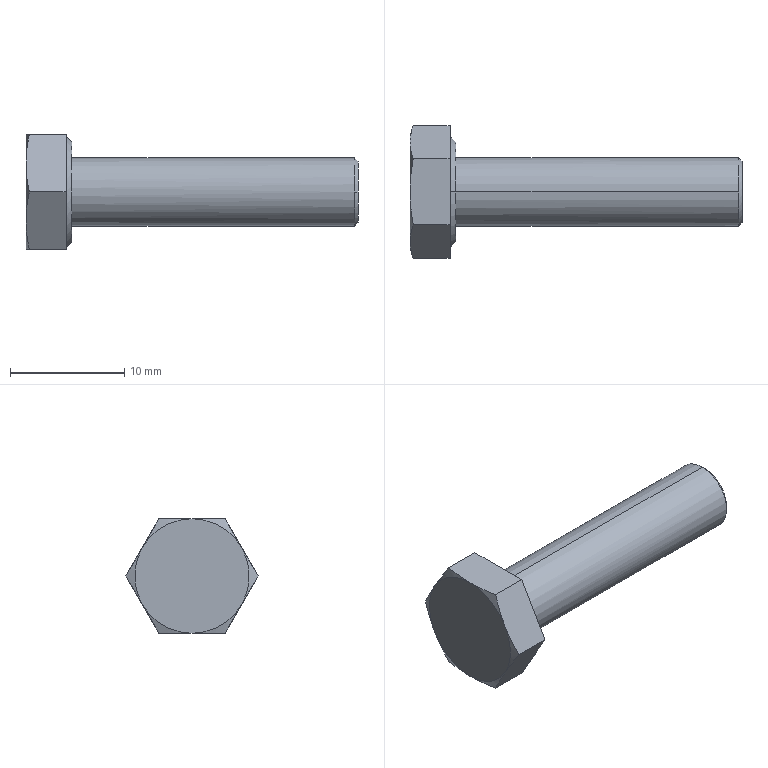Part | STEP file | hex head bolts-full thread grade c gb_GB_FASTENER_BOLT_HHBFTC M6X25-S | 1 solid | 22 faces | box 29 x 11.547 x 10 mm | volume 1042 mm3 | cone 10 | plane 10 | cylinder 2 | commonest cylinder face diameters 6 x2
STEP:
#1=CARTESIAN_POINT('',(28.7,3.,0.));
#2=VERTEX_POINT('',#1);
#3=CARTESIAN_POINT('',(28.7,0.,-3.));
#4=VERTEX_POINT('',#3);
#5=CARTESIAN_POINT('',(28.7,0.,0.));
#6=DIRECTION('',(-1.,0.,0.));
#7=DIRECTION('',(0.,0.,1.));
#8=AXIS2_PLACEMENT_3D('',#5,#6,#7);
#9=CIRCLE('',#8,3.);
#10=EDGE_CURVE('',#2,#4,#9,.T.);
#11=ORIENTED_EDGE('',*,*,#10,.T.);
#12=CARTESIAN_POINT('',(4.,0.,-3.));
#13=VERTEX_POINT('',#12);
#14=CARTESIAN_POINT('',(29.,0.,-3.));
#15=DIRECTION('',(-1.,0.,0.));
#16=VECTOR('',#15,1000.);
#17=LINE('',#14,#16);
#18=EDGE_CURVE('',#4,#13,#17,.T.);
#19=ORIENTED_EDGE('',*,*,#18,.T.);
#20=CARTESIAN_POINT('',(4.,0.,3.));
#21=VERTEX_POINT('',#20);
#22=CARTESIAN_POINT('',(4.,0.,0.));
#23=DIRECTION('',(1.,0.,0.));
#24=DIRECTION('',(0.,0.,1.));
#25=AXIS2_PLACEMENT_3D('',#22,#23,#24);
#26=CIRCLE('',#25,3.);
#27=EDGE_CURVE('',#13,#21,#26,.T.);
#28=ORIENTED_EDGE('',*,*,#27,.T.);
#29=CARTESIAN_POINT('',(28.7,0.,3.));
#30=VERTEX_POINT('',#29);
#31=CARTESIAN_POINT('',(29.,0.,3.));
#32=DIRECTION('',(-1.,0.,0.));
#33=VECTOR('',#32,1000.);
#34=LINE('',#31,#33);
#35=EDGE_CURVE('',#30,#21,#34,.T.);
#36=ORIENTED_EDGE('',*,*,#35,.F.);
#37=CARTESIAN_POINT('',(28.7,0.,0.));
#38=DIRECTION('',(-1.,0.,0.));
#39=DIRECTION('',(0.,0.,1.));
#40=AXIS2_PLACEMENT_3D('',#37,#38,#39);
#41=CIRCLE('',#40,3.);
#42=EDGE_CURVE('',#30,#2,#41,.T.);
#43=ORIENTED_EDGE('',*,*,#42,.T.);
#44=EDGE_LOOP('',(#11,#19,#28,#36,#43));
#45=FACE_OUTER_BOUND('',#44,.T.);
#46=CARTESIAN_POINT('',(29.,0.,0.));
#47=DIRECTION('',(-1.,0.,0.));
#48=DIRECTION('',(0.,0.,1.));
#49=AXIS2_PLACEMENT_3D('',#46,#47,#48);
#50=CYLINDRICAL_SURFACE('',#49,3.);
#51=ADVANCED_FACE('',(#45),#50,.T.);
#52=CARTESIAN_POINT('',(29.,-2.7,0.));
#53=VERTEX_POINT('',#52);
#54=CARTESIAN_POINT('',(29.,2.7,0.));
#55=VERTEX_POINT('',#54);
#56=CARTESIAN_POINT('',(29.,0.,0.));
#57=DIRECTION('',(-1.,0.,0.));
#58=DIRECTION('',(0.,-1.,0.));
#59=AXIS2_PLACEMENT_3D('',#56,#57,#58);
#60=CIRCLE('',#59,2.7);
#61=EDGE_CURVE('',#53,#55,#60,.T.);
#62=ORIENTED_EDGE('',*,*,#61,.T.);
#63=CARTESIAN_POINT('',(28.7,3.,0.));
#64=DIRECTION('',(-0.7071,0.7071,0.));
#65=VECTOR('',#64,1000.);
#66=LINE('',#63,#65);
#67=EDGE_CURVE('',#55,#2,#66,.T.);
#68=ORIENTED_EDGE('',*,*,#67,.T.);
#69=ORIENTED_EDGE('',*,*,#42,.F.);
#70=CARTESIAN_POINT('',(28.7,-3.,0.));
#71=VERTEX_POINT('',#70);
#72=CARTESIAN_POINT('',(28.7,0.,0.));
#73=DIRECTION('',(-1.,0.,0.));
#74=DIRECTION('',(0.,0.,1.));
#75=AXIS2_PLACEMENT_3D('',#72,#73,#74);
#76=CIRCLE('',#75,3.);
#77=EDGE_CURVE('',#71,#30,#76,.T.);
#78=ORIENTED_EDGE('',*,*,#77,.F.);
#79=CARTESIAN_POINT('',(28.7,-3.,0.));
#80=DIRECTION('',(-0.7071,-0.7071,0.));
#81=VECTOR('',#80,1000.);
#82=LINE('',#79,#81);
#83=EDGE_CURVE('',#53,#71,#82,.T.);
#84=ORIENTED_EDGE('',*,*,#83,.F.);
#85=EDGE_LOOP('',(#62,#68,#69,#78,#84));
#86=FACE_OUTER_BOUND('',#85,.T.);
#87=CARTESIAN_POINT('',(28.7,0.,0.));
#88=DIRECTION('',(-1.,0.,0.));
#89=DIRECTION('',(0.,-1.,0.));
#90=AXIS2_PLACEMENT_3D('',#87,#88,#89);
#91=CONICAL_SURFACE('',#90,3.,0.7854);
#92=ADVANCED_FACE('',(#86),#91,.T.);
#93=CARTESIAN_POINT('',(4.,0.,4.37));
#94=VERTEX_POINT('',#93);
#95=CARTESIAN_POINT('',(4.,0.,-4.37));
#96=VERTEX_POINT('',#95);
#97=CARTESIAN_POINT('',(4.,0.,0.));
#98=DIRECTION('',(-1.,0.,0.));
#99=DIRECTION('',(0.,0.,1.));
#100=AXIS2_PLACEMENT_3D('',#97,#98,#99);
#101=CIRCLE('',#100,4.37);
#102=EDGE_CURVE('',#94,#96,#101,.T.);
#103=ORIENTED_EDGE('',*,*,#102,.T.);
#104=CARTESIAN_POINT('',(3.5,0.,-4.87));
#105=VERTEX_POINT('',#104);
#106=CARTESIAN_POINT('',(3.5,0.,-4.87));
#107=DIRECTION('',(-0.7071,0.,-0.7071));
#108=VECTOR('',#107,1000.);
#109=LINE('',#106,#108);
#110=EDGE_CURVE('',#96,#105,#109,.T.);
#111=ORIENTED_EDGE('',*,*,#110,.T.);
#112=CARTESIAN_POINT('',(3.5,0.,4.87));
#113=VERTEX_POINT('',#112);
#114=CARTESIAN_POINT('',(3.5,0.,0.));
#115=DIRECTION('',(1.,0.,0.));
#116=DIRECTION('',(0.,0.,1.));
#117=AXIS2_PLACEMENT_3D('',#114,#115,#116);
#118=CIRCLE('',#117,4.87);
#119=EDGE_CURVE('',#105,#113,#118,.T.);
#120=ORIENTED_EDGE('',*,*,#119,.T.);
#121=CARTESIAN_POINT('',(3.5,0.,4.87));
#122=DIRECTION('',(-0.7071,0.,0.7071));
#123=VECTOR('',#122,1000.);
#124=LINE('',#121,#123);
#125=EDGE_CURVE('',#94,#113,#124,.T.);
#126=ORIENTED_EDGE('',*,*,#125,.F.);
#127=EDGE_LOOP('',(#103,#111,#120,#126));
#128=FACE_OUTER_BOUND('',#127,.T.);
#129=CARTESIAN_POINT('',(3.5,0.,0.));
#130=DIRECTION('',(-1.,0.,0.));
#131=DIRECTION('',(0.,0.,1.));
#132=AXIS2_PLACEMENT_3D('',#129,#130,#131);
#133=CONICAL_SURFACE('',#132,4.87,0.7854);
#134=ADVANCED_FACE('',(#128),#133,.T.);
#135=ORIENTED_EDGE('',*,*,#18,.F.);
#136=CARTESIAN_POINT('',(28.7,0.,0.));
#137=DIRECTION('',(-1.,0.,0.));
#138=DIRECTION('',(0.,0.,1.));
#139=AXIS2_PLACEMENT_3D('',#136,#137,#138);
#140=CIRCLE('',#139,3.);
#141=EDGE_CURVE('',#4,#71,#140,.T.);
#142=ORIENTED_EDGE('',*,*,#141,.T.);
#143=ORIENTED_EDGE('',*,*,#77,.T.);
#144=ORIENTED_EDGE('',*,*,#35,.T.);
#145=CARTESIAN_POINT('',(4.,0.,0.));
#146=DIRECTION('',(1.,0.,0.));
#147=DIRECTION('',(0.,0.,1.));
#148=AXIS2_PLACEMENT_3D('',#145,#146,#147);
#149=CIRCLE('',#148,3.);
#150=EDGE_CURVE('',#21,#13,#149,.T.);
#151=ORIENTED_EDGE('',*,*,#150,.T.);
#152=EDGE_LOOP('',(#135,#142,#143,#144,#151));
#153=FACE_OUTER_BOUND('',#152,.T.);
#154=CARTESIAN_POINT('',(29.,0.,0.));
#155=DIRECTION('',(-1.,0.,0.));
#156=DIRECTION('',(0.,0.,1.));
#157=AXIS2_PLACEMENT_3D('',#154,#155,#156);
#158=CYLINDRICAL_SURFACE('',#157,3.);
#159=ADVANCED_FACE('',(#153),#158,.T.);
#160=ORIENTED_EDGE('',*,*,#150,.F.);
#161=ORIENTED_EDGE('',*,*,#27,.F.);
#162=EDGE_LOOP('',(#160,#161));
#163=FACE_BOUND('',#162,.T.);
#164=ORIENTED_EDGE('',*,*,#102,.F.);
#165=CARTESIAN_POINT('',(4.,0.,0.));
#166=DIRECTION('',(-1.,0.,0.));
#167=DIRECTION('',(0.,0.,1.));
#168=AXIS2_PLACEMENT_3D('',#165,#166,#167);
#169=CIRCLE('',#168,4.37);
#170=EDGE_CURVE('',#96,#94,#169,.T.);
#171=ORIENTED_EDGE('',*,*,#170,.F.);
#172=EDGE_LOOP('',(#164,#171));
#173=FACE_OUTER_BOUND('',#172,.T.);
#174=CARTESIAN_POINT('',(4.,0.,10.));
#175=DIRECTION('',(-1.,0.,0.));
#176=DIRECTION('',(0.,0.,1.));
#177=AXIS2_PLACEMENT_3D('',#174,#175,#176);
#178=PLANE('',#177);
#179=ADVANCED_FACE('',(#163,#173),#178,.F.);
#180=ORIENTED_EDGE('',*,*,#67,.F.);
#181=CARTESIAN_POINT('',(29.,0.,0.));
#182=DIRECTION('',(-1.,0.,0.));
#183=DIRECTION('',(0.,-1.,0.));
#184=AXIS2_PLACEMENT_3D('',#181,#182,#183);
#185=CIRCLE('',#184,2.7);
#186=EDGE_CURVE('',#55,#53,#185,.T.);
#187=ORIENTED_EDGE('',*,*,#186,.T.);
#188=ORIENTED_EDGE('',*,*,#83,.T.);
#189=ORIENTED_EDGE('',*,*,#141,.F.);
#190=ORIENTED_EDGE('',*,*,#10,.F.);
#191=EDGE_LOOP('',(#180,#187,#188,#189,#190));
#192=FACE_OUTER_BOUND('',#191,.T.);
#193=CARTESIAN_POINT('',(28.7,0.,0.));
#194=DIRECTION('',(-1.,0.,0.));
#195=DIRECTION('',(0.,-1.,0.));
#196=AXIS2_PLACEMENT_3D('',#193,#194,#195);
#197=CONICAL_SURFACE('',#196,3.,0.7854);
#198=ADVANCED_FACE('',(#192),#197,.T.);
#199=ORIENTED_EDGE('',*,*,#110,.F.);
#200=ORIENTED_EDGE('',*,*,#170,.T.);
#201=ORIENTED_EDGE('',*,*,#125,.T.);
#202=CARTESIAN_POINT('',(3.5,0.,0.));
#203=DIRECTION('',(1.,0.,0.));
#204=DIRECTION('',(0.,0.,1.));
#205=AXIS2_PLACEMENT_3D('',#202,#203,#204);
#206=CIRCLE('',#205,4.87);
#207=EDGE_CURVE('',#113,#105,#206,.T.);
#208=ORIENTED_EDGE('',*,*,#207,.T.);
#209=EDGE_LOOP('',(#199,#200,#201,#208));
#210=FACE_OUTER_BOUND('',#209,.T.);
#211=CARTESIAN_POINT('',(3.5,0.,0.));
#212=DIRECTION('',(-1.,0.,0.));
#213=DIRECTION('',(0.,0.,1.));
#214=AXIS2_PLACEMENT_3D('',#211,#212,#213);
#215=CONICAL_SURFACE('',#214,4.87,0.7854);
#216=ADVANCED_FACE('',(#210),#215,.T.);
#217=ORIENTED_EDGE('',*,*,#61,.F.);
#218=ORIENTED_EDGE('',*,*,#186,.F.);
#219=EDGE_LOOP('',(#217,#218));
#220=FACE_OUTER_BOUND('',#219,.T.);
#221=CARTESIAN_POINT('',(29.,0.,0.));
#222=DIRECTION('',(1.,0.,0.));
#223=DIRECTION('',(0.,0.,-1.));
#224=AXIS2_PLACEMENT_3D('',#221,#222,#223);
#225=PLANE('',#224);
#226=ADVANCED_FACE('',(#220),#225,.T.);
#227=CARTESIAN_POINT('',(3.5,5.774,0.));
#228=VERTEX_POINT('',#227);
#229=CARTESIAN_POINT('',(3.5,2.887,5.));
#230=VERTEX_POINT('',#229);
#231=CARTESIAN_POINT('',(3.5,5.774,0.));
#232=DIRECTION('',(0.,-0.5,0.866));
#233=VECTOR('',#232,1000.);
#234=LINE('',#231,#233);
#235=EDGE_CURVE('',#228,#230,#234,.T.);
#236=ORIENTED_EDGE('',*,*,#235,.T.);
#237=CARTESIAN_POINT('',(3.5,-2.887,5.));
#238=VERTEX_POINT('',#237);
#239=CARTESIAN_POINT('',(3.5,4.87,5.));
#240=DIRECTION('',(0.,-1.,0.));
#241=VECTOR('',#240,1000.);
#242=LINE('',#239,#241);
#243=EDGE_CURVE('',#230,#238,#242,.T.);
#244=ORIENTED_EDGE('',*,*,#243,.T.);
#245=CARTESIAN_POINT('',(3.5,-5.774,0.));
#246=VERTEX_POINT('',#245);
#247=CARTESIAN_POINT('',(3.5,-2.887,5.));
#248=DIRECTION('',(0.,-0.5,-0.866));
#249=VECTOR('',#248,1000.);
#250=LINE('',#247,#249);
#251=EDGE_CURVE('',#238,#246,#250,.T.);
#252=ORIENTED_EDGE('',*,*,#251,.T.);
#253=CARTESIAN_POINT('',(3.5,-2.887,-5.));
#254=VERTEX_POINT('',#253);
#255=CARTESIAN_POINT('',(3.5,-5.774,0.));
#256=DIRECTION('',(0.,0.5,-0.866));
#257=VECTOR('',#256,1000.);
#258=LINE('',#255,#257);
#259=EDGE_CURVE('',#246,#254,#258,.T.);
#260=ORIENTED_EDGE('',*,*,#259,.T.);
#261=CARTESIAN_POINT('',(3.5,2.887,-5.));
#262=VERTEX_POINT('',#261);
#263=CARTESIAN_POINT('',(3.5,4.87,-5.));
#264=DIRECTION('',(0.,1.,0.));
#265=VECTOR('',#264,1000.);
#266=LINE('',#263,#265);
#267=EDGE_CURVE('',#254,#262,#266,.T.);
#268=ORIENTED_EDGE('',*,*,#267,.T.);
#269=CARTESIAN_POINT('',(3.5,2.887,-5.));
#270=DIRECTION('',(0.,0.5,0.866));
#271=VECTOR('',#270,1000.);
#272=LINE('',#269,#271);
#273=EDGE_CURVE('',#262,#228,#272,.T.);
#274=ORIENTED_EDGE('',*,*,#273,.T.);
#275=EDGE_LOOP('',(#236,#244,#252,#260,#268,#274));
#276=FACE_OUTER_BOUND('',#275,.T.);
#277=ORIENTED_EDGE('',*,*,#207,.F.);
#278=ORIENTED_EDGE('',*,*,#119,.F.);
#279=EDGE_LOOP('',(#277,#278));
#280=FACE_BOUND('',#279,.T.);
#281=CARTESIAN_POINT('',(3.5,4.87,0.));
#282=DIRECTION('',(1.,0.,0.));
#283=DIRECTION('',(0.,0.,-1.));
#284=AXIS2_PLACEMENT_3D('',#281,#282,#283);
#285=PLANE('',#284);
#286=ADVANCED_FACE('',(#276,#280),#285,.T.);
#287=CARTESIAN_POINT('',(0.2815,-2.887,5.));
#288=VERTEX_POINT('',#287);
#289=CARTESIAN_POINT('',(4.,-2.887,5.));
#290=DIRECTION('',(-1.,0.,0.));
#291=VECTOR('',#290,1000.);
#292=LINE('',#289,#291);
#293=EDGE_CURVE('',#238,#288,#292,.T.);
#294=ORIENTED_EDGE('',*,*,#293,.F.);
#295=ORIENTED_EDGE('',*,*,#243,.F.);
#296=CARTESIAN_POINT('',(0.2815,2.887,5.));
#297=VERTEX_POINT('',#296);
#298=CARTESIAN_POINT('',(4.,2.887,5.));
#299=DIRECTION('',(1.,0.,0.));
#300=VECTOR('',#299,1000.);
#301=LINE('',#298,#300);
#302=EDGE_CURVE('',#297,#230,#301,.T.);
#303=ORIENTED_EDGE('',*,*,#302,.F.);
#304=CARTESIAN_POINT('',(0.,0.,5.));
#305=VERTEX_POINT('',#304);
#306=CARTESIAN_POINT('',(0.,0.,5.));
#307=CARTESIAN_POINT('',(0.,0.9714,5.));
#308=CARTESIAN_POINT('',(0.1078,1.932,5.));
#309=CARTESIAN_POINT('',(0.2815,2.887,5.));
#310=B_SPLINE_CURVE_WITH_KNOTS('',3,(#306,#307,#308,#309),.UNSPECIFIED.,.F.,.F.,(4,4),(0.,0.0029),.UNSPECIFIED.);
#311=EDGE_CURVE('',#305,#297,#310,.T.);
#312=ORIENTED_EDGE('',*,*,#311,.F.);
#313=CARTESIAN_POINT('',(0.2815,-2.887,5.));
#314=CARTESIAN_POINT('',(0.1078,-1.932,5.));
#315=CARTESIAN_POINT('',(0.,-0.9714,5.));
#316=CARTESIAN_POINT('',(0.,0.,5.));
#317=B_SPLINE_CURVE_WITH_KNOTS('',3,(#313,#314,#315,#316),.UNSPECIFIED.,.F.,.F.,(4,4),(0.,0.0029),.UNSPECIFIED.);
#318=EDGE_CURVE('',#288,#305,#317,.T.);
#319=ORIENTED_EDGE('',*,*,#318,.F.);
#320=EDGE_LOOP('',(#294,#295,#303,#312,#319));
#321=FACE_OUTER_BOUND('',#320,.T.);
#322=CARTESIAN_POINT('',(4.,2.887,5.));
#323=DIRECTION('',(0.,0.,-1.));
#324=DIRECTION('',(0.,1.,0.));
#325=AXIS2_PLACEMENT_3D('',#322,#323,#324);
#326=PLANE('',#325);
#327=ADVANCED_FACE('',(#321),#326,.F.);
#328=ORIENTED_EDGE('',*,*,#302,.T.);
#329=ORIENTED_EDGE('',*,*,#235,.F.);
#330=CARTESIAN_POINT('',(0.2815,5.774,0.));
#331=VERTEX_POINT('',#330);
#332=CARTESIAN_POINT('',(4.,5.774,0.));
#333=DIRECTION('',(1.,0.,0.));
#334=VECTOR('',#333,1000.);
#335=LINE('',#332,#334);
#336=EDGE_CURVE('',#331,#228,#335,.T.);
#337=ORIENTED_EDGE('',*,*,#336,.F.);
#338=CARTESIAN_POINT('',(0.,4.33,2.5));
#339=VERTEX_POINT('',#338);
#340=CARTESIAN_POINT('',(0.,4.33,2.5));
#341=CARTESIAN_POINT('',(0.,4.816,1.659));
#342=CARTESIAN_POINT('',(0.1078,5.296,0.8266));
#343=CARTESIAN_POINT('',(0.2815,5.774,0.));
#344=B_SPLINE_CURVE_WITH_KNOTS('',3,(#340,#341,#342,#343),.UNSPECIFIED.,.F.,.F.,(4,4),(0.,0.0029),.UNSPECIFIED.);
#345=EDGE_CURVE('',#339,#331,#344,.T.);
#346=ORIENTED_EDGE('',*,*,#345,.F.);
#347=CARTESIAN_POINT('',(0.2815,2.887,5.));
#348=CARTESIAN_POINT('',(0.1078,3.364,4.173));
#349=CARTESIAN_POINT('',(0.,3.844,3.341));
#350=CARTESIAN_POINT('',(0.,4.33,2.5));
#351=B_SPLINE_CURVE_WITH_KNOTS('',3,(#347,#348,#349,#350),.UNSPECIFIED.,.F.,.F.,(4,4),(0.,0.0029),.UNSPECIFIED.);
#352=EDGE_CURVE('',#297,#339,#351,.T.);
#353=ORIENTED_EDGE('',*,*,#352,.F.);
#354=EDGE_LOOP('',(#328,#329,#337,#346,#353));
#355=FACE_OUTER_BOUND('',#354,.T.);
#356=CARTESIAN_POINT('',(4.,5.774,0.));
#357=DIRECTION('',(0.,-0.866,-0.5));
#358=DIRECTION('',(0.,0.5,-0.866));
#359=AXIS2_PLACEMENT_3D('',#356,#357,#358);
#360=PLANE('',#359);
#361=ADVANCED_FACE('',(#355),#360,.F.);
#362=ORIENTED_EDGE('',*,*,#336,.T.);
#363=ORIENTED_EDGE('',*,*,#273,.F.);
#364=CARTESIAN_POINT('',(0.2815,2.887,-5.));
#365=VERTEX_POINT('',#364);
#366=CARTESIAN_POINT('',(4.,2.887,-5.));
#367=DIRECTION('',(1.,0.,0.));
#368=VECTOR('',#367,1000.);
#369=LINE('',#366,#368);
#370=EDGE_CURVE('',#365,#262,#369,.T.);
#371=ORIENTED_EDGE('',*,*,#370,.F.);
#372=CARTESIAN_POINT('',(0.,4.33,-2.5));
#373=VERTEX_POINT('',#372);
#374=CARTESIAN_POINT('',(0.,4.33,-2.5));
#375=CARTESIAN_POINT('',(0.,3.844,-3.341));
#376=CARTESIAN_POINT('',(0.1078,3.364,-4.173));
#377=CARTESIAN_POINT('',(0.2815,2.887,-5.));
#378=B_SPLINE_CURVE_WITH_KNOTS('',3,(#374,#375,#376,#377),.UNSPECIFIED.,.F.,.F.,(4,4),(0.,0.0029),.UNSPECIFIED.);
#379=EDGE_CURVE('',#373,#365,#378,.T.);
#380=ORIENTED_EDGE('',*,*,#379,.F.);
#381=CARTESIAN_POINT('',(0.2815,5.774,0.));
#382=CARTESIAN_POINT('',(0.1078,5.296,-0.8266));
#383=CARTESIAN_POINT('',(0.,4.816,-1.659));
#384=CARTESIAN_POINT('',(0.,4.33,-2.5));
#385=B_SPLINE_CURVE_WITH_KNOTS('',3,(#381,#382,#383,#384),.UNSPECIFIED.,.F.,.F.,(4,4),(0.,0.0029),.UNSPECIFIED.);
#386=EDGE_CURVE('',#331,#373,#385,.T.);
#387=ORIENTED_EDGE('',*,*,#386,.F.);
#388=EDGE_LOOP('',(#362,#363,#371,#380,#387));
#389=FACE_OUTER_BOUND('',#388,.T.);
#390=CARTESIAN_POINT('',(4.,2.887,-5.));
#391=DIRECTION('',(0.,-0.866,0.5));
#392=DIRECTION('',(0.,-0.5,-0.866));
#393=AXIS2_PLACEMENT_3D('',#390,#391,#392);
#394=PLANE('',#393);
#395=ADVANCED_FACE('',(#389),#394,.F.);
#396=ORIENTED_EDGE('',*,*,#370,.T.);
#397=ORIENTED_EDGE('',*,*,#267,.F.);
#398=CARTESIAN_POINT('',(0.2815,-2.887,-5.));
#399=VERTEX_POINT('',#398);
#400=CARTESIAN_POINT('',(4.,-2.887,-5.));
#401=DIRECTION('',(1.,0.,0.));
#402=VECTOR('',#401,1000.);
#403=LINE('',#400,#402);
#404=EDGE_CURVE('',#399,#254,#403,.T.);
#405=ORIENTED_EDGE('',*,*,#404,.F.);
#406=CARTESIAN_POINT('',(0.,0.,-5.));
#407=VERTEX_POINT('',#406);
#408=CARTESIAN_POINT('',(0.,0.,-5.));
#409=CARTESIAN_POINT('',(0.,-0.9714,-5.));
#410=CARTESIAN_POINT('',(0.1078,-1.932,-5.));
#411=CARTESIAN_POINT('',(0.2815,-2.887,-5.));
#412=B_SPLINE_CURVE_WITH_KNOTS('',3,(#408,#409,#410,#411),.UNSPECIFIED.,.F.,.F.,(4,4),(0.,0.0029),.UNSPECIFIED.);
#413=EDGE_CURVE('',#407,#399,#412,.T.);
#414=ORIENTED_EDGE('',*,*,#413,.F.);
#415=CARTESIAN_POINT('',(0.2815,2.887,-5.));
#416=CARTESIAN_POINT('',(0.1078,1.932,-5.));
#417=CARTESIAN_POINT('',(0.,0.9714,-5.));
#418=CARTESIAN_POINT('',(0.,0.,-5.));
#419=B_SPLINE_CURVE_WITH_KNOTS('',3,(#415,#416,#417,#418),.UNSPECIFIED.,.F.,.F.,(4,4),(0.,0.0029),.UNSPECIFIED.);
#420=EDGE_CURVE('',#365,#407,#419,.T.);
#421=ORIENTED_EDGE('',*,*,#420,.F.);
#422=EDGE_LOOP('',(#396,#397,#405,#414,#421));
#423=FACE_OUTER_BOUND('',#422,.T.);
#424=CARTESIAN_POINT('',(4.,-2.887,-5.));
#425=DIRECTION('',(0.,0.,1.));
#426=DIRECTION('',(1.,0.,0.));
#427=AXIS2_PLACEMENT_3D('',#424,#425,#426);
#428=PLANE('',#427);
#429=ADVANCED_FACE('',(#423),#428,.F.);
#430=ORIENTED_EDGE('',*,*,#404,.T.);
#431=ORIENTED_EDGE('',*,*,#259,.F.);
#432=CARTESIAN_POINT('',(0.2815,-5.774,0.));
#433=VERTEX_POINT('',#432);
#434=CARTESIAN_POINT('',(4.,-5.774,0.));
#435=DIRECTION('',(1.,0.,0.));
#436=VECTOR('',#435,1000.);
#437=LINE('',#434,#436);
#438=EDGE_CURVE('',#433,#246,#437,.T.);
#439=ORIENTED_EDGE('',*,*,#438,.F.);
#440=CARTESIAN_POINT('',(0.,-4.33,-2.5));
#441=VERTEX_POINT('',#440);
#442=CARTESIAN_POINT('',(0.,-4.33,-2.5));
#443=CARTESIAN_POINT('',(0.,-4.816,-1.659));
#444=CARTESIAN_POINT('',(0.1078,-5.296,-0.8266));
#445=CARTESIAN_POINT('',(0.2815,-5.774,0.));
#446=B_SPLINE_CURVE_WITH_KNOTS('',3,(#442,#443,#444,#445),.UNSPECIFIED.,.F.,.F.,(4,4),(0.,0.0029),.UNSPECIFIED.);
#447=EDGE_CURVE('',#441,#433,#446,.T.);
#448=ORIENTED_EDGE('',*,*,#447,.F.);
#449=CARTESIAN_POINT('',(0.2815,-2.887,-5.));
#450=CARTESIAN_POINT('',(0.1078,-3.364,-4.173));
#451=CARTESIAN_POINT('',(0.,-3.844,-3.341));
#452=CARTESIAN_POINT('',(0.,-4.33,-2.5));
#453=B_SPLINE_CURVE_WITH_KNOTS('',3,(#449,#450,#451,#452),.UNSPECIFIED.,.F.,.F.,(4,4),(0.,0.0029),.UNSPECIFIED.);
#454=EDGE_CURVE('',#399,#441,#453,.T.);
#455=ORIENTED_EDGE('',*,*,#454,.F.);
#456=EDGE_LOOP('',(#430,#431,#439,#448,#455));
#457=FACE_OUTER_BOUND('',#456,.T.);
#458=CARTESIAN_POINT('',(4.,-5.774,0.));
#459=DIRECTION('',(0.,0.866,0.5));
#460=DIRECTION('',(0.,-0.5,0.866));
#461=AXIS2_PLACEMENT_3D('',#458,#459,#460);
#462=PLANE('',#461);
#463=ADVANCED_FACE('',(#457),#462,.F.);
#464=ORIENTED_EDGE('',*,*,#438,.T.);
#465=ORIENTED_EDGE('',*,*,#251,.F.);
#466=ORIENTED_EDGE('',*,*,#293,.T.);
#467=CARTESIAN_POINT('',(0.,-4.33,2.5));
#468=VERTEX_POINT('',#467);
#469=CARTESIAN_POINT('',(0.,-4.33,2.5));
#470=CARTESIAN_POINT('',(0.,-3.844,3.341));
#471=CARTESIAN_POINT('',(0.1078,-3.364,4.173));
#472=CARTESIAN_POINT('',(0.2815,-2.887,5.));
#473=B_SPLINE_CURVE_WITH_KNOTS('',3,(#469,#470,#471,#472),.UNSPECIFIED.,.F.,.F.,(4,4),(0.,0.0029),.UNSPECIFIED.);
#474=EDGE_CURVE('',#468,#288,#473,.T.);
#475=ORIENTED_EDGE('',*,*,#474,.F.);
#476=CARTESIAN_POINT('',(0.2815,-5.774,0.));
#477=CARTESIAN_POINT('',(0.1078,-5.296,0.8266));
#478=CARTESIAN_POINT('',(0.,-4.816,1.659));
#479=CARTESIAN_POINT('',(0.,-4.33,2.5));
#480=B_SPLINE_CURVE_WITH_KNOTS('',3,(#476,#477,#478,#479),.UNSPECIFIED.,.F.,.F.,(4,4),(0.,0.0029),.UNSPECIFIED.);
#481=EDGE_CURVE('',#433,#468,#480,.T.);
#482=ORIENTED_EDGE('',*,*,#481,.F.);
#483=EDGE_LOOP('',(#464,#465,#466,#475,#482));
#484=FACE_OUTER_BOUND('',#483,.T.);
#485=CARTESIAN_POINT('',(4.,-2.887,5.));
#486=DIRECTION('',(0.,0.866,-0.5));
#487=DIRECTION('',(0.,0.5,0.866));
#488=AXIS2_PLACEMENT_3D('',#485,#486,#487);
#489=PLANE('',#488);
#490=ADVANCED_FACE('',(#484),#489,.F.);
#491=ORIENTED_EDGE('',*,*,#318,.T.);
#492=CARTESIAN_POINT('',(0.,0.,0.));
#493=DIRECTION('',(1.,0.,0.));
#494=DIRECTION('',(0.,0.,-1.));
#495=AXIS2_PLACEMENT_3D('',#492,#493,#494);
#496=CIRCLE('',#495,5.);
#497=EDGE_CURVE('',#305,#468,#496,.T.);
#498=ORIENTED_EDGE('',*,*,#497,.T.);
#499=ORIENTED_EDGE('',*,*,#474,.T.);
#500=EDGE_LOOP('',(#491,#498,#499));
#501=FACE_OUTER_BOUND('',#500,.T.);
#502=CARTESIAN_POINT('',(0.2832,0.,0.));
#503=DIRECTION('',(1.,0.,0.));
#504=DIRECTION('',(0.,0.,-1.));
#505=AXIS2_PLACEMENT_3D('',#502,#503,#504);
#506=CONICAL_SURFACE('',#505,5.778,1.222);
#507=ADVANCED_FACE('',(#501),#506,.T.);
#508=CARTESIAN_POINT('',(0.,0.,0.));
#509=DIRECTION('',(1.,0.,0.));
#510=DIRECTION('',(0.,0.,-1.));
#511=AXIS2_PLACEMENT_3D('',#508,#509,#510);
#512=CIRCLE('',#511,5.);
#513=EDGE_CURVE('',#339,#305,#512,.T.);
#514=ORIENTED_EDGE('',*,*,#513,.T.);
#515=ORIENTED_EDGE('',*,*,#311,.T.);
#516=ORIENTED_EDGE('',*,*,#352,.T.);
#517=EDGE_LOOP('',(#514,#515,#516));
#518=FACE_OUTER_BOUND('',#517,.T.);
#519=CARTESIAN_POINT('',(0.2832,0.,0.));
#520=DIRECTION('',(1.,0.,0.));
#521=DIRECTION('',(0.,0.,-1.));
#522=AXIS2_PLACEMENT_3D('',#519,#520,#521);
#523=CONICAL_SURFACE('',#522,5.778,1.222);
#524=ADVANCED_FACE('',(#518),#523,.T.);
#525=CARTESIAN_POINT('',(0.,0.,0.));
#526=DIRECTION('',(1.,0.,0.));
#527=DIRECTION('',(0.,0.,-1.));
#528=AXIS2_PLACEMENT_3D('',#525,#526,#527);
#529=CIRCLE('',#528,5.);
#530=EDGE_CURVE('',#373,#339,#529,.T.);
#531=ORIENTED_EDGE('',*,*,#530,.T.);
#532=ORIENTED_EDGE('',*,*,#345,.T.);
#533=ORIENTED_EDGE('',*,*,#386,.T.);
#534=EDGE_LOOP('',(#531,#532,#533));
#535=FACE_OUTER_BOUND('',#534,.T.);
#536=CARTESIAN_POINT('',(0.2832,0.,0.));
#537=DIRECTION('',(1.,0.,0.));
#538=DIRECTION('',(0.,0.,-1.));
#539=AXIS2_PLACEMENT_3D('',#536,#537,#538);
#540=CONICAL_SURFACE('',#539,5.778,1.222);
#541=ADVANCED_FACE('',(#535),#540,.T.);
#542=CARTESIAN_POINT('',(0.,0.,0.));
#543=DIRECTION('',(1.,0.,0.));
#544=DIRECTION('',(0.,0.,-1.));
#545=AXIS2_PLACEMENT_3D('',#542,#543,#544);
#546=CIRCLE('',#545,5.);
#547=EDGE_CURVE('',#407,#373,#546,.T.);
#548=ORIENTED_EDGE('',*,*,#547,.T.);
#549=ORIENTED_EDGE('',*,*,#379,.T.);
#550=ORIENTED_EDGE('',*,*,#420,.T.);
#551=EDGE_LOOP('',(#548,#549,#550));
#552=FACE_OUTER_BOUND('',#551,.T.);
#553=CARTESIAN_POINT('',(0.2832,0.,0.));
#554=DIRECTION('',(1.,0.,0.));
#555=DIRECTION('',(0.,0.,-1.));
#556=AXIS2_PLACEMENT_3D('',#553,#554,#555);
#557=CONICAL_SURFACE('',#556,5.778,1.222);
#558=ADVANCED_FACE('',(#552),#557,.T.);
#559=ORIENTED_EDGE('',*,*,#454,.T.);
#560=CARTESIAN_POINT('',(0.,0.,0.));
#561=DIRECTION('',(1.,0.,0.));
#562=DIRECTION('',(0.,0.,-1.));
#563=AXIS2_PLACEMENT_3D('',#560,#561,#562);
#564=CIRCLE('',#563,5.);
#565=EDGE_CURVE('',#441,#407,#564,.T.);
#566=ORIENTED_EDGE('',*,*,#565,.T.);
#567=ORIENTED_EDGE('',*,*,#413,.T.);
#568=EDGE_LOOP('',(#559,#566,#567));
#569=FACE_OUTER_BOUND('',#568,.T.);
#570=CARTESIAN_POINT('',(0.2832,0.,0.));
#571=DIRECTION('',(1.,0.,0.));
#572=DIRECTION('',(0.,0.,-1.));
#573=AXIS2_PLACEMENT_3D('',#570,#571,#572);
#574=CONICAL_SURFACE('',#573,5.778,1.222);
#575=ADVANCED_FACE('',(#569),#574,.T.);
#576=ORIENTED_EDGE('',*,*,#481,.T.);
#577=CARTESIAN_POINT('',(0.,0.,0.));
#578=DIRECTION('',(1.,0.,0.));
#579=DIRECTION('',(0.,0.,-1.));
#580=AXIS2_PLACEMENT_3D('',#577,#578,#579);
#581=CIRCLE('',#580,5.);
#582=EDGE_CURVE('',#468,#441,#581,.T.);
#583=ORIENTED_EDGE('',*,*,#582,.T.);
#584=ORIENTED_EDGE('',*,*,#447,.T.);
#585=EDGE_LOOP('',(#576,#583,#584));
#586=FACE_OUTER_BOUND('',#585,.T.);
#587=CARTESIAN_POINT('',(0.2832,0.,0.));
#588=DIRECTION('',(1.,0.,0.));
#589=DIRECTION('',(0.,0.,-1.));
#590=AXIS2_PLACEMENT_3D('',#587,#588,#589);
#591=CONICAL_SURFACE('',#590,5.778,1.222);
#592=ADVANCED_FACE('',(#586),#591,.T.);
#593=ORIENTED_EDGE('',*,*,#565,.F.);
#594=ORIENTED_EDGE('',*,*,#582,.F.);
#595=ORIENTED_EDGE('',*,*,#497,.F.);
#596=ORIENTED_EDGE('',*,*,#513,.F.);
#597=ORIENTED_EDGE('',*,*,#530,.F.);
#598=ORIENTED_EDGE('',*,*,#547,.F.);
#599=EDGE_LOOP('',(#593,#594,#595,#596,#597,#598));
#600=FACE_OUTER_BOUND('',#599,.T.);
#601=CARTESIAN_POINT('',(0.,0.,10.));
#602=DIRECTION('',(-1.,0.,0.));
#603=DIRECTION('',(0.,0.,1.));
#604=AXIS2_PLACEMENT_3D('',#601,#602,#603);
#605=PLANE('',#604);
#606=ADVANCED_FACE('',(#600),#605,.T.);
#607=CLOSED_SHELL('',(#51,#92,#134,#159,#179,#198,#216,#226,#286,#327,#361,#395,#429,#463,#490,#507,#524,#541,#558,#575,#592,#606));
#608=MANIFOLD_SOLID_BREP('',#607);
#609=CARTESIAN_POINT('',(0.,0.,0.));
#610=DIRECTION('',(0.,0.,1.));
#611=DIRECTION('',(1.,0.,0.));
#612=AXIS2_PLACEMENT_3D('',#609,#610,#611);
#613=(LENGTH_UNIT()NAMED_UNIT(*)SI_UNIT(.MILLI.,.METRE.));
#614=UNCERTAINTY_MEASURE_WITH_UNIT(LENGTH_MEASURE(0.00001),#613,'','');
#615=(NAMED_UNIT(*)PLANE_ANGLE_UNIT()SI_UNIT($,.RADIAN.));
#616=(NAMED_UNIT(*)SI_UNIT($,.STERADIAN.)SOLID_ANGLE_UNIT());
#617=(GEOMETRIC_REPRESENTATION_CONTEXT(3)GLOBAL_UNCERTAINTY_ASSIGNED_CONTEXT((#614))GLOBAL_UNIT_ASSIGNED_CONTEXT((#613,#615,#616))REPRESENTATION_CONTEXT('',''));
#618=ADVANCED_BREP_SHAPE_REPRESENTATION('',(#608,#612),#617);